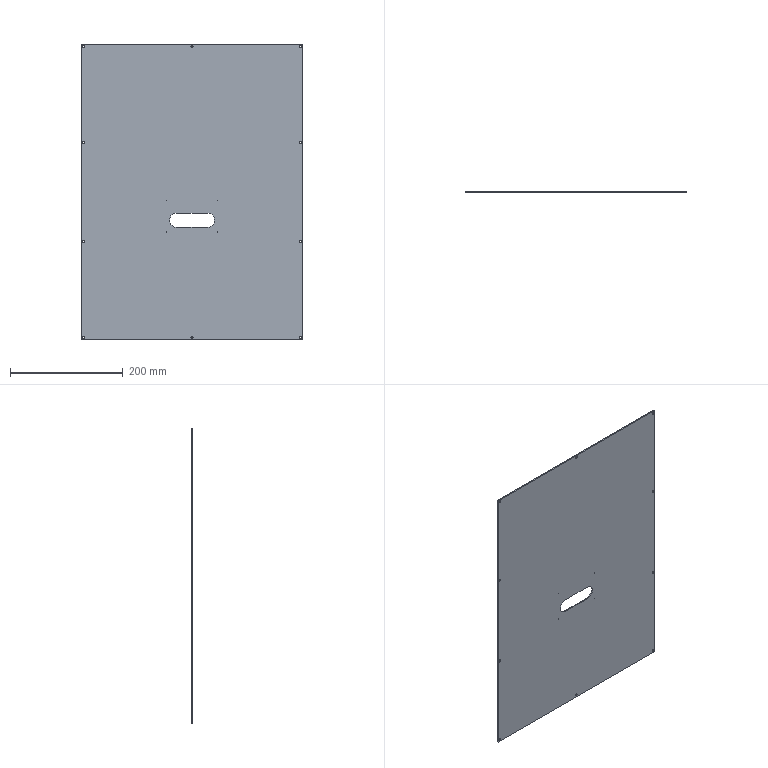Part | NX | features solid 2 | 1 solid | 39 faces | box 393 x 2 x 524 mm | volume 407875 mm3 | cylinder 31 | plane 8 | commonest cylinder face diameters 4 x20 1 x8 25 x3
STEP:
#1=CARTESIAN_POINT('',(-708.,-1585.,647.));
#2=VERTEX_POINT('',#1);
#3=CARTESIAN_POINT('',(-708.,-1587.,647.));
#4=VERTEX_POINT('',#3);
#5=CARTESIAN_POINT('',(-708.,-931.997,647.));
#6=DIRECTION('',(0.,-1.,0.));
#7=VECTOR('',#6,1000.);
#8=LINE('',#5,#7);
#9=EDGE_CURVE('',#2,#4,#8,.T.);
#10=ORIENTED_EDGE('',*,*,#9,.F.);
#11=CARTESIAN_POINT('',(-707.,-1585.,647.));
#12=VERTEX_POINT('',#11);
#13=CARTESIAN_POINT('',(-707.5,-1585.,647.));
#14=DIRECTION('',(0.,-1.,0.));
#15=DIRECTION('',(1.,0.,0.));
#16=AXIS2_PLACEMENT_3D('',#13,#14,#15);
#17=CIRCLE('',#16,0.5);
#18=EDGE_CURVE('',#12,#2,#17,.T.);
#19=ORIENTED_EDGE('',*,*,#18,.F.);
#20=CARTESIAN_POINT('',(-707.,-1587.,647.));
#21=VERTEX_POINT('',#20);
#22=CARTESIAN_POINT('',(-707.,-931.997,647.));
#23=DIRECTION('',(0.,-1.,0.));
#24=VECTOR('',#23,1000.);
#25=LINE('',#22,#24);
#26=EDGE_CURVE('',#21,#12,#25,.F.);
#27=ORIENTED_EDGE('',*,*,#26,.F.);
#28=CARTESIAN_POINT('',(-707.5,-1587.,647.));
#29=DIRECTION('',(0.,-1.,0.));
#30=DIRECTION('',(1.,0.,0.));
#31=AXIS2_PLACEMENT_3D('',#28,#29,#30);
#32=CIRCLE('',#31,0.5);
#33=EDGE_CURVE('',#21,#4,#32,.T.);
#34=ORIENTED_EDGE('',*,*,#33,.T.);
#35=EDGE_LOOP('',(#10,#19,#27,#34));
#36=FACE_BOUND('',#35,.T.);
#37=CARTESIAN_POINT('',(-707.5,-931.997,647.));
#38=DIRECTION('',(0.,-1.,0.));
#39=DIRECTION('',(1.,0.,0.));
#40=AXIS2_PLACEMENT_3D('',#37,#38,#39);
#41=CYLINDRICAL_SURFACE('',#40,0.5);
#42=ADVANCED_FACE('',(#36),#41,.F.);
#43=CARTESIAN_POINT('',(-618.,-1585.,647.));
#44=VERTEX_POINT('',#43);
#45=CARTESIAN_POINT('',(-618.,-1587.,647.));
#46=VERTEX_POINT('',#45);
#47=CARTESIAN_POINT('',(-618.,-931.997,647.));
#48=DIRECTION('',(0.,-1.,0.));
#49=VECTOR('',#48,1000.);
#50=LINE('',#47,#49);
#51=EDGE_CURVE('',#44,#46,#50,.T.);
#52=ORIENTED_EDGE('',*,*,#51,.F.);
#53=CARTESIAN_POINT('',(-617.,-1585.,647.));
#54=VERTEX_POINT('',#53);
#55=CARTESIAN_POINT('',(-617.5,-1585.,647.));
#56=DIRECTION('',(0.,-1.,0.));
#57=DIRECTION('',(1.,0.,0.));
#58=AXIS2_PLACEMENT_3D('',#55,#56,#57);
#59=CIRCLE('',#58,0.5);
#60=EDGE_CURVE('',#54,#44,#59,.T.);
#61=ORIENTED_EDGE('',*,*,#60,.F.);
#62=CARTESIAN_POINT('',(-617.,-1587.,647.));
#63=VERTEX_POINT('',#62);
#64=CARTESIAN_POINT('',(-617.,-931.997,647.));
#65=DIRECTION('',(0.,-1.,0.));
#66=VECTOR('',#65,1000.);
#67=LINE('',#64,#66);
#68=EDGE_CURVE('',#63,#54,#67,.F.);
#69=ORIENTED_EDGE('',*,*,#68,.F.);
#70=CARTESIAN_POINT('',(-617.5,-1587.,647.));
#71=DIRECTION('',(0.,-1.,0.));
#72=DIRECTION('',(1.,0.,0.));
#73=AXIS2_PLACEMENT_3D('',#70,#71,#72);
#74=CIRCLE('',#73,0.5);
#75=EDGE_CURVE('',#63,#46,#74,.T.);
#76=ORIENTED_EDGE('',*,*,#75,.T.);
#77=EDGE_LOOP('',(#52,#61,#69,#76));
#78=FACE_BOUND('',#77,.T.);
#79=CARTESIAN_POINT('',(-617.5,-931.997,647.));
#80=DIRECTION('',(0.,-1.,0.));
#81=DIRECTION('',(1.,0.,0.));
#82=AXIS2_PLACEMENT_3D('',#79,#80,#81);
#83=CYLINDRICAL_SURFACE('',#82,0.5);
#84=ADVANCED_FACE('',(#78),#83,.F.);
#85=CARTESIAN_POINT('',(-618.,-1587.,591.));
#86=VERTEX_POINT('',#85);
#87=CARTESIAN_POINT('',(-618.,-1585.,591.));
#88=VERTEX_POINT('',#87);
#89=CARTESIAN_POINT('',(-618.,-931.997,591.));
#90=DIRECTION('',(0.,-1.,0.));
#91=VECTOR('',#90,1000.);
#92=LINE('',#89,#91);
#93=EDGE_CURVE('',#86,#88,#92,.F.);
#94=ORIENTED_EDGE('',*,*,#93,.T.);
#95=CARTESIAN_POINT('',(-617.,-1585.,591.));
#96=VERTEX_POINT('',#95);
#97=CARTESIAN_POINT('',(-617.5,-1585.,591.));
#98=DIRECTION('',(0.,-1.,0.));
#99=DIRECTION('',(1.,0.,0.));
#100=AXIS2_PLACEMENT_3D('',#97,#98,#99);
#101=CIRCLE('',#100,0.5);
#102=EDGE_CURVE('',#96,#88,#101,.T.);
#103=ORIENTED_EDGE('',*,*,#102,.F.);
#104=CARTESIAN_POINT('',(-617.,-1587.,591.));
#105=VERTEX_POINT('',#104);
#106=CARTESIAN_POINT('',(-617.,-931.997,591.));
#107=DIRECTION('',(0.,-1.,0.));
#108=VECTOR('',#107,1000.);
#109=LINE('',#106,#108);
#110=EDGE_CURVE('',#96,#105,#109,.T.);
#111=ORIENTED_EDGE('',*,*,#110,.T.);
#112=CARTESIAN_POINT('',(-617.5,-1587.,591.));
#113=DIRECTION('',(0.,-1.,0.));
#114=DIRECTION('',(1.,0.,0.));
#115=AXIS2_PLACEMENT_3D('',#112,#113,#114);
#116=CIRCLE('',#115,0.5);
#117=EDGE_CURVE('',#105,#86,#116,.T.);
#118=ORIENTED_EDGE('',*,*,#117,.T.);
#119=EDGE_LOOP('',(#94,#103,#111,#118));
#120=FACE_BOUND('',#119,.T.);
#121=CARTESIAN_POINT('',(-617.5,-931.997,591.));
#122=DIRECTION('',(0.,-1.,0.));
#123=DIRECTION('',(1.,0.,0.));
#124=AXIS2_PLACEMENT_3D('',#121,#122,#123);
#125=CYLINDRICAL_SURFACE('',#124,0.5);
#126=ADVANCED_FACE('',(#120),#125,.F.);
#127=CARTESIAN_POINT('',(-708.,-1587.,591.));
#128=VERTEX_POINT('',#127);
#129=CARTESIAN_POINT('',(-708.,-1585.,591.));
#130=VERTEX_POINT('',#129);
#131=CARTESIAN_POINT('',(-708.,-931.997,591.));
#132=DIRECTION('',(0.,-1.,0.));
#133=VECTOR('',#132,1000.);
#134=LINE('',#131,#133);
#135=EDGE_CURVE('',#128,#130,#134,.F.);
#136=ORIENTED_EDGE('',*,*,#135,.T.);
#137=CARTESIAN_POINT('',(-707.,-1585.,591.));
#138=VERTEX_POINT('',#137);
#139=CARTESIAN_POINT('',(-707.5,-1585.,591.));
#140=DIRECTION('',(0.,-1.,0.));
#141=DIRECTION('',(1.,0.,0.));
#142=AXIS2_PLACEMENT_3D('',#139,#140,#141);
#143=CIRCLE('',#142,0.5);
#144=EDGE_CURVE('',#138,#130,#143,.T.);
#145=ORIENTED_EDGE('',*,*,#144,.F.);
#146=CARTESIAN_POINT('',(-707.,-1587.,591.));
#147=VERTEX_POINT('',#146);
#148=CARTESIAN_POINT('',(-707.,-931.997,591.));
#149=DIRECTION('',(0.,-1.,0.));
#150=VECTOR('',#149,1000.);
#151=LINE('',#148,#150);
#152=EDGE_CURVE('',#138,#147,#151,.T.);
#153=ORIENTED_EDGE('',*,*,#152,.T.);
#154=CARTESIAN_POINT('',(-707.5,-1587.,591.));
#155=DIRECTION('',(0.,-1.,0.));
#156=DIRECTION('',(1.,0.,0.));
#157=AXIS2_PLACEMENT_3D('',#154,#155,#156);
#158=CIRCLE('',#157,0.5);
#159=EDGE_CURVE('',#147,#128,#158,.T.);
#160=ORIENTED_EDGE('',*,*,#159,.T.);
#161=EDGE_LOOP('',(#136,#145,#153,#160));
#162=FACE_BOUND('',#161,.T.);
#163=CARTESIAN_POINT('',(-707.5,-931.997,591.));
#164=DIRECTION('',(0.,-1.,0.));
#165=DIRECTION('',(1.,0.,0.));
#166=AXIS2_PLACEMENT_3D('',#163,#164,#165);
#167=CYLINDRICAL_SURFACE('',#166,0.5);
#168=ADVANCED_FACE('',(#162),#167,.F.);
#169=CARTESIAN_POINT('',(-690.,-1587.,599.5));
#170=VERTEX_POINT('',#169);
#171=CARTESIAN_POINT('',(-635.,-1587.,599.5));
#172=VERTEX_POINT('',#171);
#173=CARTESIAN_POINT('',(-859.,-1587.,599.5));
#174=DIRECTION('',(1.,0.,0.));
#175=VECTOR('',#174,1000.);
#176=LINE('',#173,#175);
#177=EDGE_CURVE('',#170,#172,#176,.T.);
#178=ORIENTED_EDGE('',*,*,#177,.T.);
#179=CARTESIAN_POINT('',(-635.,-1585.,599.5));
#180=VERTEX_POINT('',#179);
#181=CARTESIAN_POINT('',(-635.,-2240.003,599.5));
#182=DIRECTION('',(0.,1.,0.));
#183=VECTOR('',#182,1000.);
#184=LINE('',#181,#183);
#185=EDGE_CURVE('',#172,#180,#184,.T.);
#186=ORIENTED_EDGE('',*,*,#185,.T.);
#187=CARTESIAN_POINT('',(-690.,-1585.,599.5));
#188=VERTEX_POINT('',#187);
#189=CARTESIAN_POINT('',(-635.,-1585.,599.5));
#190=DIRECTION('',(-1.,0.,0.));
#191=VECTOR('',#190,1000.);
#192=LINE('',#189,#191);
#193=EDGE_CURVE('',#180,#188,#192,.T.);
#194=ORIENTED_EDGE('',*,*,#193,.T.);
#195=CARTESIAN_POINT('',(-690.,-2240.003,599.5));
#196=DIRECTION('',(0.,1.,0.));
#197=VECTOR('',#196,1000.);
#198=LINE('',#195,#197);
#199=EDGE_CURVE('',#170,#188,#198,.T.);
#200=ORIENTED_EDGE('',*,*,#199,.F.);
#201=EDGE_LOOP('',(#178,#186,#194,#200));
#202=FACE_BOUND('',#201,.T.);
#203=CARTESIAN_POINT('',(-635.,-2240.003,599.5));
#204=DIRECTION('',(0.,0.,-1.));
#205=DIRECTION('',(0.,-1.,0.));
#206=AXIS2_PLACEMENT_3D('',#203,#204,#205);
#207=PLANE('',#206);
#208=ADVANCED_FACE('',(#202),#207,.F.);
#209=CARTESIAN_POINT('',(-635.,-1587.,624.5));
#210=VERTEX_POINT('',#209);
#211=CARTESIAN_POINT('',(-635.,-1587.,612.));
#212=DIRECTION('',(0.,-1.,0.));
#213=DIRECTION('',(1.,0.,0.));
#214=AXIS2_PLACEMENT_3D('',#211,#212,#213);
#215=CIRCLE('',#214,12.5);
#216=EDGE_CURVE('',#172,#210,#215,.T.);
#217=ORIENTED_EDGE('',*,*,#216,.T.);
#218=CARTESIAN_POINT('',(-635.,-1585.,624.5));
#219=VERTEX_POINT('',#218);
#220=CARTESIAN_POINT('',(-635.,-2240.003,624.5));
#221=DIRECTION('',(0.,1.,0.));
#222=VECTOR('',#221,1000.);
#223=LINE('',#220,#222);
#224=EDGE_CURVE('',#210,#219,#223,.T.);
#225=ORIENTED_EDGE('',*,*,#224,.T.);
#226=CARTESIAN_POINT('',(-635.,-1585.,612.));
#227=DIRECTION('',(0.,1.,0.));
#228=DIRECTION('',(-1.,0.,0.));
#229=AXIS2_PLACEMENT_3D('',#226,#227,#228);
#230=CIRCLE('',#229,12.5);
#231=EDGE_CURVE('',#219,#180,#230,.T.);
#232=ORIENTED_EDGE('',*,*,#231,.T.);
#233=ORIENTED_EDGE('',*,*,#185,.F.);
#234=EDGE_LOOP('',(#217,#225,#232,#233));
#235=FACE_BOUND('',#234,.T.);
#236=CARTESIAN_POINT('',(-635.,-2240.003,612.));
#237=DIRECTION('',(0.,1.,0.));
#238=DIRECTION('',(-1.,0.,0.));
#239=AXIS2_PLACEMENT_3D('',#236,#237,#238);
#240=CYLINDRICAL_SURFACE('',#239,12.5);
#241=ADVANCED_FACE('',(#235),#240,.F.);
#242=CARTESIAN_POINT('',(-690.,-1587.,624.5));
#243=VERTEX_POINT('',#242);
#244=CARTESIAN_POINT('',(-859.,-1587.,624.5));
#245=DIRECTION('',(-1.,0.,0.));
#246=VECTOR('',#245,1000.);
#247=LINE('',#244,#246);
#248=EDGE_CURVE('',#210,#243,#247,.T.);
#249=ORIENTED_EDGE('',*,*,#248,.T.);
#250=CARTESIAN_POINT('',(-690.,-1585.,624.5));
#251=VERTEX_POINT('',#250);
#252=CARTESIAN_POINT('',(-690.,-2240.003,624.5));
#253=DIRECTION('',(0.,1.,0.));
#254=VECTOR('',#253,1000.);
#255=LINE('',#252,#254);
#256=EDGE_CURVE('',#243,#251,#255,.T.);
#257=ORIENTED_EDGE('',*,*,#256,.T.);
#258=CARTESIAN_POINT('',(-635.,-1585.,624.5));
#259=DIRECTION('',(1.,0.,0.));
#260=VECTOR('',#259,1000.);
#261=LINE('',#258,#260);
#262=EDGE_CURVE('',#251,#219,#261,.T.);
#263=ORIENTED_EDGE('',*,*,#262,.T.);
#264=ORIENTED_EDGE('',*,*,#224,.F.);
#265=EDGE_LOOP('',(#249,#257,#263,#264));
#266=FACE_BOUND('',#265,.T.);
#267=CARTESIAN_POINT('',(-635.,-2240.003,624.5));
#268=DIRECTION('',(0.,0.,1.));
#269=DIRECTION('',(1.,0.,0.));
#270=AXIS2_PLACEMENT_3D('',#267,#268,#269);
#271=PLANE('',#270);
#272=ADVANCED_FACE('',(#266),#271,.F.);
#273=CARTESIAN_POINT('',(-702.5,-1587.,612.));
#274=VERTEX_POINT('',#273);
#275=CARTESIAN_POINT('',(-702.5,-1585.,612.));
#276=VERTEX_POINT('',#275);
#277=CARTESIAN_POINT('',(-702.5,-2240.003,612.));
#278=DIRECTION('',(0.,1.,0.));
#279=VECTOR('',#278,1000.);
#280=LINE('',#277,#279);
#281=EDGE_CURVE('',#274,#276,#280,.T.);
#282=ORIENTED_EDGE('',*,*,#281,.F.);
#283=CARTESIAN_POINT('',(-690.,-1587.,612.));
#284=DIRECTION('',(0.,-1.,0.));
#285=DIRECTION('',(1.,0.,0.));
#286=AXIS2_PLACEMENT_3D('',#283,#284,#285);
#287=CIRCLE('',#286,12.5);
#288=EDGE_CURVE('',#274,#170,#287,.T.);
#289=ORIENTED_EDGE('',*,*,#288,.T.);
#290=ORIENTED_EDGE('',*,*,#199,.T.);
#291=CARTESIAN_POINT('',(-690.,-1585.,612.));
#292=DIRECTION('',(0.,1.,0.));
#293=DIRECTION('',(1.,0.,0.));
#294=AXIS2_PLACEMENT_3D('',#291,#292,#293);
#295=CIRCLE('',#294,12.5);
#296=EDGE_CURVE('',#188,#276,#295,.T.);
#297=ORIENTED_EDGE('',*,*,#296,.T.);
#298=EDGE_LOOP('',(#282,#289,#290,#297));
#299=FACE_BOUND('',#298,.T.);
#300=CARTESIAN_POINT('',(-690.,-2240.003,612.));
#301=DIRECTION('',(0.,1.,0.));
#302=DIRECTION('',(-1.,0.,0.));
#303=AXIS2_PLACEMENT_3D('',#300,#301,#302);
#304=CYLINDRICAL_SURFACE('',#303,12.5);
#305=ADVANCED_FACE('',(#299),#304,.F.);
#306=CARTESIAN_POINT('',(-472.,-1585.,574.));
#307=VERTEX_POINT('',#306);
#308=CARTESIAN_POINT('',(-472.,-1587.,574.));
#309=VERTEX_POINT('',#308);
#310=CARTESIAN_POINT('',(-472.,-931.997,574.));
#311=DIRECTION('',(0.,-1.,0.));
#312=VECTOR('',#311,1000.);
#313=LINE('',#310,#312);
#314=EDGE_CURVE('',#307,#309,#313,.T.);
#315=ORIENTED_EDGE('',*,*,#314,.F.);
#316=CARTESIAN_POINT('',(-468.,-1585.,574.));
#317=VERTEX_POINT('',#316);
#318=CARTESIAN_POINT('',(-470.,-1585.,574.));
#319=DIRECTION('',(0.,-1.,0.));
#320=DIRECTION('',(1.,0.,0.));
#321=AXIS2_PLACEMENT_3D('',#318,#319,#320);
#322=CIRCLE('',#321,2.);
#323=EDGE_CURVE('',#317,#307,#322,.T.);
#324=ORIENTED_EDGE('',*,*,#323,.F.);
#325=CARTESIAN_POINT('',(-468.,-1587.,574.));
#326=VERTEX_POINT('',#325);
#327=CARTESIAN_POINT('',(-468.,-931.997,574.));
#328=DIRECTION('',(0.,-1.,0.));
#329=VECTOR('',#328,1000.);
#330=LINE('',#327,#329);
#331=EDGE_CURVE('',#326,#317,#330,.F.);
#332=ORIENTED_EDGE('',*,*,#331,.F.);
#333=CARTESIAN_POINT('',(-470.,-1587.,574.));
#334=DIRECTION('',(0.,-1.,0.));
#335=DIRECTION('',(1.,0.,0.));
#336=AXIS2_PLACEMENT_3D('',#333,#334,#335);
#337=CIRCLE('',#336,2.);
#338=EDGE_CURVE('',#326,#309,#337,.T.);
#339=ORIENTED_EDGE('',*,*,#338,.T.);
#340=EDGE_LOOP('',(#315,#324,#332,#339));
#341=FACE_BOUND('',#340,.T.);
#342=CARTESIAN_POINT('',(-470.,-931.997,574.));
#343=DIRECTION('',(0.,-1.,0.));
#344=DIRECTION('',(1.,0.,0.));
#345=AXIS2_PLACEMENT_3D('',#342,#343,#344);
#346=CYLINDRICAL_SURFACE('',#345,2.);
#347=ADVANCED_FACE('',(#341),#346,.F.);
#348=CARTESIAN_POINT('',(-857.,-1587.,574.));
#349=VERTEX_POINT('',#348);
#350=CARTESIAN_POINT('',(-857.,-1585.,574.));
#351=VERTEX_POINT('',#350);
#352=CARTESIAN_POINT('',(-857.,-931.997,574.));
#353=DIRECTION('',(0.,-1.,0.));
#354=VECTOR('',#353,1000.);
#355=LINE('',#352,#354);
#356=EDGE_CURVE('',#349,#351,#355,.F.);
#357=ORIENTED_EDGE('',*,*,#356,.T.);
#358=CARTESIAN_POINT('',(-853.,-1585.,574.));
#359=VERTEX_POINT('',#358);
#360=CARTESIAN_POINT('',(-855.,-1585.,574.));
#361=DIRECTION('',(0.,-1.,0.));
#362=DIRECTION('',(1.,0.,0.));
#363=AXIS2_PLACEMENT_3D('',#360,#361,#362);
#364=CIRCLE('',#363,2.);
#365=EDGE_CURVE('',#359,#351,#364,.T.);
#366=ORIENTED_EDGE('',*,*,#365,.F.);
#367=CARTESIAN_POINT('',(-853.,-1587.,574.));
#368=VERTEX_POINT('',#367);
#369=CARTESIAN_POINT('',(-853.,-931.997,574.));
#370=DIRECTION('',(0.,-1.,0.));
#371=VECTOR('',#370,1000.);
#372=LINE('',#369,#371);
#373=EDGE_CURVE('',#359,#368,#372,.T.);
#374=ORIENTED_EDGE('',*,*,#373,.T.);
#375=CARTESIAN_POINT('',(-855.,-1587.,574.));
#376=DIRECTION('',(0.,-1.,0.));
#377=DIRECTION('',(1.,0.,0.));
#378=AXIS2_PLACEMENT_3D('',#375,#376,#377);
#379=CIRCLE('',#378,2.);
#380=EDGE_CURVE('',#368,#349,#379,.T.);
#381=ORIENTED_EDGE('',*,*,#380,.T.);
#382=EDGE_LOOP('',(#357,#366,#374,#381));
#383=FACE_BOUND('',#382,.T.);
#384=CARTESIAN_POINT('',(-855.,-931.997,574.));
#385=DIRECTION('',(0.,-1.,0.));
#386=DIRECTION('',(1.,0.,0.));
#387=AXIS2_PLACEMENT_3D('',#384,#385,#386);
#388=CYLINDRICAL_SURFACE('',#387,2.);
#389=ADVANCED_FACE('',(#383),#388,.F.);
#390=CARTESIAN_POINT('',(-857.,-1587.,920.));
#391=VERTEX_POINT('',#390);
#392=CARTESIAN_POINT('',(-857.,-1585.,920.));
#393=VERTEX_POINT('',#392);
#394=CARTESIAN_POINT('',(-857.,-931.997,920.));
#395=DIRECTION('',(0.,-1.,0.));
#396=VECTOR('',#395,1000.);
#397=LINE('',#394,#396);
#398=EDGE_CURVE('',#391,#393,#397,.F.);
#399=ORIENTED_EDGE('',*,*,#398,.T.);
#400=CARTESIAN_POINT('',(-853.,-1585.,920.));
#401=VERTEX_POINT('',#400);
#402=CARTESIAN_POINT('',(-855.,-1585.,920.));
#403=DIRECTION('',(0.,-1.,0.));
#404=DIRECTION('',(1.,0.,0.));
#405=AXIS2_PLACEMENT_3D('',#402,#403,#404);
#406=CIRCLE('',#405,2.);
#407=EDGE_CURVE('',#401,#393,#406,.T.);
#408=ORIENTED_EDGE('',*,*,#407,.F.);
#409=CARTESIAN_POINT('',(-853.,-1587.,920.));
#410=VERTEX_POINT('',#409);
#411=CARTESIAN_POINT('',(-853.,-931.997,920.));
#412=DIRECTION('',(0.,-1.,0.));
#413=VECTOR('',#412,1000.);
#414=LINE('',#411,#413);
#415=EDGE_CURVE('',#401,#410,#414,.T.);
#416=ORIENTED_EDGE('',*,*,#415,.T.);
#417=CARTESIAN_POINT('',(-855.,-1587.,920.));
#418=DIRECTION('',(0.,-1.,0.));
#419=DIRECTION('',(1.,0.,0.));
#420=AXIS2_PLACEMENT_3D('',#417,#418,#419);
#421=CIRCLE('',#420,2.);
#422=EDGE_CURVE('',#410,#391,#421,.T.);
#423=ORIENTED_EDGE('',*,*,#422,.T.);
#424=EDGE_LOOP('',(#399,#408,#416,#423));
#425=FACE_BOUND('',#424,.T.);
#426=CARTESIAN_POINT('',(-855.,-931.997,920.));
#427=DIRECTION('',(0.,-1.,0.));
#428=DIRECTION('',(1.,0.,0.));
#429=AXIS2_PLACEMENT_3D('',#426,#427,#428);
#430=CYLINDRICAL_SURFACE('',#429,2.);
#431=ADVANCED_FACE('',(#425),#430,.F.);
#432=CARTESIAN_POINT('',(-857.,-1585.,750.));
#433=VERTEX_POINT('',#432);
#434=CARTESIAN_POINT('',(-857.,-1587.,750.));
#435=VERTEX_POINT('',#434);
#436=CARTESIAN_POINT('',(-857.,-931.997,750.));
#437=DIRECTION('',(0.,-1.,0.));
#438=VECTOR('',#437,1000.);
#439=LINE('',#436,#438);
#440=EDGE_CURVE('',#433,#435,#439,.T.);
#441=ORIENTED_EDGE('',*,*,#440,.F.);
#442=CARTESIAN_POINT('',(-853.,-1585.,750.));
#443=VERTEX_POINT('',#442);
#444=CARTESIAN_POINT('',(-855.,-1585.,750.));
#445=DIRECTION('',(0.,-1.,0.));
#446=DIRECTION('',(1.,0.,0.));
#447=AXIS2_PLACEMENT_3D('',#444,#445,#446);
#448=CIRCLE('',#447,2.);
#449=EDGE_CURVE('',#443,#433,#448,.T.);
#450=ORIENTED_EDGE('',*,*,#449,.F.);
#451=CARTESIAN_POINT('',(-853.,-1587.,750.));
#452=VERTEX_POINT('',#451);
#453=CARTESIAN_POINT('',(-853.,-931.997,750.));
#454=DIRECTION('',(0.,-1.,0.));
#455=VECTOR('',#454,1000.);
#456=LINE('',#453,#455);
#457=EDGE_CURVE('',#452,#443,#456,.F.);
#458=ORIENTED_EDGE('',*,*,#457,.F.);
#459=CARTESIAN_POINT('',(-855.,-1587.,750.));
#460=DIRECTION('',(0.,-1.,0.));
#461=DIRECTION('',(1.,0.,0.));
#462=AXIS2_PLACEMENT_3D('',#459,#460,#461);
#463=CIRCLE('',#462,2.);
#464=EDGE_CURVE('',#452,#435,#463,.T.);
#465=ORIENTED_EDGE('',*,*,#464,.T.);
#466=EDGE_LOOP('',(#441,#450,#458,#465));
#467=FACE_BOUND('',#466,.T.);
#468=CARTESIAN_POINT('',(-855.,-931.997,750.));
#469=DIRECTION('',(0.,-1.,0.));
#470=DIRECTION('',(1.,0.,0.));
#471=AXIS2_PLACEMENT_3D('',#468,#469,#470);
#472=CYLINDRICAL_SURFACE('',#471,2.);
#473=ADVANCED_FACE('',(#467),#472,.F.);
#474=CARTESIAN_POINT('',(-857.,-1587.,404.));
#475=VERTEX_POINT('',#474);
#476=CARTESIAN_POINT('',(-857.,-1585.,404.));
#477=VERTEX_POINT('',#476);
#478=CARTESIAN_POINT('',(-857.,-931.997,404.));
#479=DIRECTION('',(0.,-1.,0.));
#480=VECTOR('',#479,1000.);
#481=LINE('',#478,#480);
#482=EDGE_CURVE('',#475,#477,#481,.F.);
#483=ORIENTED_EDGE('',*,*,#482,.T.);
#484=CARTESIAN_POINT('',(-853.,-1585.,404.));
#485=VERTEX_POINT('',#484);
#486=CARTESIAN_POINT('',(-855.,-1585.,404.));
#487=DIRECTION('',(0.,-1.,0.));
#488=DIRECTION('',(1.,0.,0.));
#489=AXIS2_PLACEMENT_3D('',#486,#487,#488);
#490=CIRCLE('',#489,2.);
#491=EDGE_CURVE('',#485,#477,#490,.T.);
#492=ORIENTED_EDGE('',*,*,#491,.F.);
#493=CARTESIAN_POINT('',(-853.,-1587.,404.));
#494=VERTEX_POINT('',#493);
#495=CARTESIAN_POINT('',(-853.,-931.997,404.));
#496=DIRECTION('',(0.,-1.,0.));
#497=VECTOR('',#496,1000.);
#498=LINE('',#495,#497);
#499=EDGE_CURVE('',#485,#494,#498,.T.);
#500=ORIENTED_EDGE('',*,*,#499,.T.);
#501=CARTESIAN_POINT('',(-855.,-1587.,404.));
#502=DIRECTION('',(0.,-1.,0.));
#503=DIRECTION('',(1.,0.,0.));
#504=AXIS2_PLACEMENT_3D('',#501,#502,#503);
#505=CIRCLE('',#504,2.);
#506=EDGE_CURVE('',#494,#475,#505,.T.);
#507=ORIENTED_EDGE('',*,*,#506,.T.);
#508=EDGE_LOOP('',(#483,#492,#500,#507));
#509=FACE_BOUND('',#508,.T.);
#510=CARTESIAN_POINT('',(-855.,-931.997,404.));
#511=DIRECTION('',(0.,-1.,0.));
#512=DIRECTION('',(1.,0.,0.));
#513=AXIS2_PLACEMENT_3D('',#510,#511,#512);
#514=CYLINDRICAL_SURFACE('',#513,2.);
#515=ADVANCED_FACE('',(#509),#514,.F.);
#516=CARTESIAN_POINT('',(-664.5,-1587.,404.));
#517=VERTEX_POINT('',#516);
#518=CARTESIAN_POINT('',(-664.5,-1585.,404.));
#519=VERTEX_POINT('',#518);
#520=CARTESIAN_POINT('',(-664.5,-931.997,404.));
#521=DIRECTION('',(0.,-1.,0.));
#522=VECTOR('',#521,1000.);
#523=LINE('',#520,#522);
#524=EDGE_CURVE('',#517,#519,#523,.F.);
#525=ORIENTED_EDGE('',*,*,#524,.T.);
#526=CARTESIAN_POINT('',(-660.5,-1585.,404.));
#527=VERTEX_POINT('',#526);
#528=CARTESIAN_POINT('',(-662.5,-1585.,404.));
#529=DIRECTION('',(0.,-1.,0.));
#530=DIRECTION('',(1.,0.,0.));
#531=AXIS2_PLACEMENT_3D('',#528,#529,#530);
#532=CIRCLE('',#531,2.);
#533=EDGE_CURVE('',#527,#519,#532,.T.);
#534=ORIENTED_EDGE('',*,*,#533,.F.);
#535=CARTESIAN_POINT('',(-660.5,-1587.,404.));
#536=VERTEX_POINT('',#535);
#537=CARTESIAN_POINT('',(-660.5,-931.997,404.));
#538=DIRECTION('',(0.,-1.,0.));
#539=VECTOR('',#538,1000.);
#540=LINE('',#537,#539);
#541=EDGE_CURVE('',#527,#536,#540,.T.);
#542=ORIENTED_EDGE('',*,*,#541,.T.);
#543=CARTESIAN_POINT('',(-662.5,-1587.,404.));
#544=DIRECTION('',(0.,-1.,0.));
#545=DIRECTION('',(1.,0.,0.));
#546=AXIS2_PLACEMENT_3D('',#543,#544,#545);
#547=CIRCLE('',#546,2.);
#548=EDGE_CURVE('',#536,#517,#547,.T.);
#549=ORIENTED_EDGE('',*,*,#548,.T.);
#550=EDGE_LOOP('',(#525,#534,#542,#549));
#551=FACE_BOUND('',#550,.T.);
#552=CARTESIAN_POINT('',(-662.5,-931.997,404.));
#553=DIRECTION('',(0.,-1.,0.));
#554=DIRECTION('',(1.,0.,0.));
#555=AXIS2_PLACEMENT_3D('',#552,#553,#554);
#556=CYLINDRICAL_SURFACE('',#555,2.);
#557=ADVANCED_FACE('',(#551),#556,.F.);
#558=CARTESIAN_POINT('',(-472.,-1585.,404.));
#559=VERTEX_POINT('',#558);
#560=CARTESIAN_POINT('',(-472.,-1587.,404.));
#561=VERTEX_POINT('',#560);
#562=CARTESIAN_POINT('',(-472.,-931.997,404.));
#563=DIRECTION('',(0.,-1.,0.));
#564=VECTOR('',#563,1000.);
#565=LINE('',#562,#564);
#566=EDGE_CURVE('',#559,#561,#565,.T.);
#567=ORIENTED_EDGE('',*,*,#566,.F.);
#568=CARTESIAN_POINT('',(-468.,-1585.,404.));
#569=VERTEX_POINT('',#568);
#570=CARTESIAN_POINT('',(-470.,-1585.,404.));
#571=DIRECTION('',(0.,-1.,0.));
#572=DIRECTION('',(1.,0.,0.));
#573=AXIS2_PLACEMENT_3D('',#570,#571,#572);
#574=CIRCLE('',#573,2.);
#575=EDGE_CURVE('',#569,#559,#574,.T.);
#576=ORIENTED_EDGE('',*,*,#575,.F.);
#577=CARTESIAN_POINT('',(-468.,-1587.,404.));
#578=VERTEX_POINT('',#577);
#579=CARTESIAN_POINT('',(-468.,-931.997,404.));
#580=DIRECTION('',(0.,-1.,0.));
#581=VECTOR('',#580,1000.);
#582=LINE('',#579,#581);
#583=EDGE_CURVE('',#578,#569,#582,.F.);
#584=ORIENTED_EDGE('',*,*,#583,.F.);
#585=CARTESIAN_POINT('',(-470.,-1587.,404.));
#586=DIRECTION('',(0.,-1.,0.));
#587=DIRECTION('',(1.,0.,0.));
#588=AXIS2_PLACEMENT_3D('',#585,#586,#587);
#589=CIRCLE('',#588,2.);
#590=EDGE_CURVE('',#578,#561,#589,.T.);
#591=ORIENTED_EDGE('',*,*,#590,.T.);
#592=EDGE_LOOP('',(#567,#576,#584,#591));
#593=FACE_BOUND('',#592,.T.);
#594=CARTESIAN_POINT('',(-470.,-931.997,404.));
#595=DIRECTION('',(0.,-1.,0.));
#596=DIRECTION('',(1.,0.,0.));
#597=AXIS2_PLACEMENT_3D('',#594,#595,#596);
#598=CYLINDRICAL_SURFACE('',#597,2.);
#599=ADVANCED_FACE('',(#593),#598,.F.);
#600=CARTESIAN_POINT('',(-472.,-1585.,750.));
#601=VERTEX_POINT('',#600);
#602=CARTESIAN_POINT('',(-472.,-1587.,750.));
#603=VERTEX_POINT('',#602);
#604=CARTESIAN_POINT('',(-472.,-931.997,750.));
#605=DIRECTION('',(0.,-1.,0.));
#606=VECTOR('',#605,1000.);
#607=LINE('',#604,#606);
#608=EDGE_CURVE('',#601,#603,#607,.T.);
#609=ORIENTED_EDGE('',*,*,#608,.F.);
#610=CARTESIAN_POINT('',(-468.,-1585.,750.));
#611=VERTEX_POINT('',#610);
#612=CARTESIAN_POINT('',(-470.,-1585.,750.));
#613=DIRECTION('',(0.,-1.,0.));
#614=DIRECTION('',(1.,0.,0.));
#615=AXIS2_PLACEMENT_3D('',#612,#613,#614);
#616=CIRCLE('',#615,2.);
#617=EDGE_CURVE('',#611,#601,#616,.T.);
#618=ORIENTED_EDGE('',*,*,#617,.F.);
#619=CARTESIAN_POINT('',(-468.,-1587.,750.));
#620=VERTEX_POINT('',#619);
#621=CARTESIAN_POINT('',(-468.,-931.997,750.));
#622=DIRECTION('',(0.,-1.,0.));
#623=VECTOR('',#622,1000.);
#624=LINE('',#621,#623);
#625=EDGE_CURVE('',#620,#611,#624,.F.);
#626=ORIENTED_EDGE('',*,*,#625,.F.);
#627=CARTESIAN_POINT('',(-470.,-1587.,750.));
#628=DIRECTION('',(0.,-1.,0.));
#629=DIRECTION('',(1.,0.,0.));
#630=AXIS2_PLACEMENT_3D('',#627,#628,#629);
#631=CIRCLE('',#630,2.);
#632=EDGE_CURVE('',#620,#603,#631,.T.);
#633=ORIENTED_EDGE('',*,*,#632,.T.);
#634=EDGE_LOOP('',(#609,#618,#626,#633));
#635=FACE_BOUND('',#634,.T.);
#636=CARTESIAN_POINT('',(-470.,-931.997,750.));
#637=DIRECTION('',(0.,-1.,0.));
#638=DIRECTION('',(1.,0.,0.));
#639=AXIS2_PLACEMENT_3D('',#636,#637,#638);
#640=CYLINDRICAL_SURFACE('',#639,2.);
#641=ADVANCED_FACE('',(#635),#640,.F.);
#642=CARTESIAN_POINT('',(-472.,-1585.,920.));
#643=VERTEX_POINT('',#642);
#644=CARTESIAN_POINT('',(-472.,-1587.,920.));
#645=VERTEX_POINT('',#644);
#646=CARTESIAN_POINT('',(-472.,-931.997,920.));
#647=DIRECTION('',(0.,-1.,0.));
#648=VECTOR('',#647,1000.);
#649=LINE('',#646,#648);
#650=EDGE_CURVE('',#643,#645,#649,.T.);
#651=ORIENTED_EDGE('',*,*,#650,.F.);
#652=CARTESIAN_POINT('',(-468.,-1585.,920.));
#653=VERTEX_POINT('',#652);
#654=CARTESIAN_POINT('',(-470.,-1585.,920.));
#655=DIRECTION('',(0.,-1.,0.));
#656=DIRECTION('',(1.,0.,0.));
#657=AXIS2_PLACEMENT_3D('',#654,#655,#656);
#658=CIRCLE('',#657,2.);
#659=EDGE_CURVE('',#653,#643,#658,.T.);
#660=ORIENTED_EDGE('',*,*,#659,.F.);
#661=CARTESIAN_POINT('',(-468.,-1587.,920.));
#662=VERTEX_POINT('',#661);
#663=CARTESIAN_POINT('',(-468.,-931.997,920.));
#664=DIRECTION('',(0.,-1.,0.));
#665=VECTOR('',#664,1000.);
#666=LINE('',#663,#665);
#667=EDGE_CURVE('',#662,#653,#666,.F.);
#668=ORIENTED_EDGE('',*,*,#667,.F.);
#669=CARTESIAN_POINT('',(-470.,-1587.,920.));
#670=DIRECTION('',(0.,-1.,0.));
#671=DIRECTION('',(1.,0.,0.));
#672=AXIS2_PLACEMENT_3D('',#669,#670,#671);
#673=CIRCLE('',#672,2.);
#674=EDGE_CURVE('',#662,#645,#673,.T.);
#675=ORIENTED_EDGE('',*,*,#674,.T.);
#676=EDGE_LOOP('',(#651,#660,#668,#675));
#677=FACE_BOUND('',#676,.T.);
#678=CARTESIAN_POINT('',(-470.,-931.997,920.));
#679=DIRECTION('',(0.,-1.,0.));
#680=DIRECTION('',(1.,0.,0.));
#681=AXIS2_PLACEMENT_3D('',#678,#679,#680);
#682=CYLINDRICAL_SURFACE('',#681,2.);
#683=ADVANCED_FACE('',(#677),#682,.F.);
#684=CARTESIAN_POINT('',(-664.5,-1585.,920.));
#685=VERTEX_POINT('',#684);
#686=CARTESIAN_POINT('',(-664.5,-1587.,920.));
#687=VERTEX_POINT('',#686);
#688=CARTESIAN_POINT('',(-664.5,-931.997,920.));
#689=DIRECTION('',(0.,-1.,0.));
#690=VECTOR('',#689,1000.);
#691=LINE('',#688,#690);
#692=EDGE_CURVE('',#685,#687,#691,.T.);
#693=ORIENTED_EDGE('',*,*,#692,.F.);
#694=CARTESIAN_POINT('',(-660.5,-1585.,920.));
#695=VERTEX_POINT('',#694);
#696=CARTESIAN_POINT('',(-662.5,-1585.,920.));
#697=DIRECTION('',(0.,-1.,0.));
#698=DIRECTION('',(1.,0.,0.));
#699=AXIS2_PLACEMENT_3D('',#696,#697,#698);
#700=CIRCLE('',#699,2.);
#701=EDGE_CURVE('',#695,#685,#700,.T.);
#702=ORIENTED_EDGE('',*,*,#701,.F.);
#703=CARTESIAN_POINT('',(-660.5,-1587.,920.));
#704=VERTEX_POINT('',#703);
#705=CARTESIAN_POINT('',(-660.5,-931.997,920.));
#706=DIRECTION('',(0.,-1.,0.));
#707=VECTOR('',#706,1000.);
#708=LINE('',#705,#707);
#709=EDGE_CURVE('',#704,#695,#708,.F.);
#710=ORIENTED_EDGE('',*,*,#709,.F.);
#711=CARTESIAN_POINT('',(-662.5,-1587.,920.));
#712=DIRECTION('',(0.,-1.,0.));
#713=DIRECTION('',(1.,0.,0.));
#714=AXIS2_PLACEMENT_3D('',#711,#712,#713);
#715=CIRCLE('',#714,2.);
#716=EDGE_CURVE('',#704,#687,#715,.T.);
#717=ORIENTED_EDGE('',*,*,#716,.T.);
#718=EDGE_LOOP('',(#693,#702,#710,#717));
#719=FACE_BOUND('',#718,.T.);
#720=CARTESIAN_POINT('',(-662.5,-931.997,920.));
#721=DIRECTION('',(0.,-1.,0.));
#722=DIRECTION('',(1.,0.,0.));
#723=AXIS2_PLACEMENT_3D('',#720,#721,#722);
#724=CYLINDRICAL_SURFACE('',#723,2.);
#725=ADVANCED_FACE('',(#719),#724,.F.);
#726=ORIENTED_EDGE('',*,*,#701,.T.);
#727=CARTESIAN_POINT('',(-662.5,-1585.,920.));
#728=DIRECTION('',(0.,-1.,0.));
#729=DIRECTION('',(1.,0.,0.));
#730=AXIS2_PLACEMENT_3D('',#727,#728,#729);
#731=CIRCLE('',#730,2.);
#732=EDGE_CURVE('',#685,#695,#731,.T.);
#733=ORIENTED_EDGE('',*,*,#732,.T.);
#734=EDGE_LOOP('',(#726,#733));
#735=FACE_BOUND('',#734,.T.);
#736=ORIENTED_EDGE('',*,*,#659,.T.);
#737=CARTESIAN_POINT('',(-470.,-1585.,920.));
#738=DIRECTION('',(0.,-1.,0.));
#739=DIRECTION('',(1.,0.,0.));
#740=AXIS2_PLACEMENT_3D('',#737,#738,#739);
#741=CIRCLE('',#740,2.);
#742=EDGE_CURVE('',#643,#653,#741,.T.);
#743=ORIENTED_EDGE('',*,*,#742,.T.);
#744=EDGE_LOOP('',(#736,#743));
#745=FACE_BOUND('',#744,.T.);
#746=ORIENTED_EDGE('',*,*,#617,.T.);
#747=CARTESIAN_POINT('',(-470.,-1585.,750.));
#748=DIRECTION('',(0.,-1.,0.));
#749=DIRECTION('',(1.,0.,0.));
#750=AXIS2_PLACEMENT_3D('',#747,#748,#749);
#751=CIRCLE('',#750,2.);
#752=EDGE_CURVE('',#601,#611,#751,.T.);
#753=ORIENTED_EDGE('',*,*,#752,.T.);
#754=EDGE_LOOP('',(#746,#753));
#755=FACE_BOUND('',#754,.T.);
#756=ORIENTED_EDGE('',*,*,#575,.T.);
#757=CARTESIAN_POINT('',(-470.,-1585.,404.));
#758=DIRECTION('',(0.,-1.,0.));
#759=DIRECTION('',(1.,0.,0.));
#760=AXIS2_PLACEMENT_3D('',#757,#758,#759);
#761=CIRCLE('',#760,2.);
#762=EDGE_CURVE('',#559,#569,#761,.T.);
#763=ORIENTED_EDGE('',*,*,#762,.T.);
#764=EDGE_LOOP('',(#756,#763));
#765=FACE_BOUND('',#764,.T.);
#766=ORIENTED_EDGE('',*,*,#533,.T.);
#767=CARTESIAN_POINT('',(-662.5,-1585.,404.));
#768=DIRECTION('',(0.,-1.,0.));
#769=DIRECTION('',(1.,0.,0.));
#770=AXIS2_PLACEMENT_3D('',#767,#768,#769);
#771=CIRCLE('',#770,2.);
#772=EDGE_CURVE('',#519,#527,#771,.T.);
#773=ORIENTED_EDGE('',*,*,#772,.T.);
#774=EDGE_LOOP('',(#766,#773));
#775=FACE_BOUND('',#774,.T.);
#776=ORIENTED_EDGE('',*,*,#491,.T.);
#777=CARTESIAN_POINT('',(-855.,-1585.,404.));
#778=DIRECTION('',(0.,-1.,0.));
#779=DIRECTION('',(1.,0.,0.));
#780=AXIS2_PLACEMENT_3D('',#777,#778,#779);
#781=CIRCLE('',#780,2.);
#782=EDGE_CURVE('',#477,#485,#781,.T.);
#783=ORIENTED_EDGE('',*,*,#782,.T.);
#784=EDGE_LOOP('',(#776,#783));
#785=FACE_BOUND('',#784,.T.);
#786=ORIENTED_EDGE('',*,*,#449,.T.);
#787=CARTESIAN_POINT('',(-855.,-1585.,750.));
#788=DIRECTION('',(0.,-1.,0.));
#789=DIRECTION('',(1.,0.,0.));
#790=AXIS2_PLACEMENT_3D('',#787,#788,#789);
#791=CIRCLE('',#790,2.);
#792=EDGE_CURVE('',#433,#443,#791,.T.);
#793=ORIENTED_EDGE('',*,*,#792,.T.);
#794=EDGE_LOOP('',(#786,#793));
#795=FACE_BOUND('',#794,.T.);
#796=ORIENTED_EDGE('',*,*,#407,.T.);
#797=CARTESIAN_POINT('',(-855.,-1585.,920.));
#798=DIRECTION('',(0.,-1.,0.));
#799=DIRECTION('',(1.,0.,0.));
#800=AXIS2_PLACEMENT_3D('',#797,#798,#799);
#801=CIRCLE('',#800,2.);
#802=EDGE_CURVE('',#393,#401,#801,.T.);
#803=ORIENTED_EDGE('',*,*,#802,.T.);
#804=EDGE_LOOP('',(#796,#803));
#805=FACE_BOUND('',#804,.T.);
#806=ORIENTED_EDGE('',*,*,#365,.T.);
#807=CARTESIAN_POINT('',(-855.,-1585.,574.));
#808=DIRECTION('',(0.,-1.,0.));
#809=DIRECTION('',(1.,0.,0.));
#810=AXIS2_PLACEMENT_3D('',#807,#808,#809);
#811=CIRCLE('',#810,2.);
#812=EDGE_CURVE('',#351,#359,#811,.T.);
#813=ORIENTED_EDGE('',*,*,#812,.T.);
#814=EDGE_LOOP('',(#806,#813));
#815=FACE_BOUND('',#814,.T.);
#816=ORIENTED_EDGE('',*,*,#323,.T.);
#817=CARTESIAN_POINT('',(-470.,-1585.,574.));
#818=DIRECTION('',(0.,-1.,0.));
#819=DIRECTION('',(1.,0.,0.));
#820=AXIS2_PLACEMENT_3D('',#817,#818,#819);
#821=CIRCLE('',#820,2.);
#822=EDGE_CURVE('',#307,#317,#821,.T.);
#823=ORIENTED_EDGE('',*,*,#822,.T.);
#824=EDGE_LOOP('',(#816,#823));
#825=FACE_BOUND('',#824,.T.);
#826=ORIENTED_EDGE('',*,*,#262,.F.);
#827=CARTESIAN_POINT('',(-690.,-1585.,612.));
#828=DIRECTION('',(0.,1.,0.));
#829=DIRECTION('',(1.,0.,0.));
#830=AXIS2_PLACEMENT_3D('',#827,#828,#829);
#831=CIRCLE('',#830,12.5);
#832=EDGE_CURVE('',#276,#251,#831,.T.);
#833=ORIENTED_EDGE('',*,*,#832,.F.);
#834=ORIENTED_EDGE('',*,*,#296,.F.);
#835=ORIENTED_EDGE('',*,*,#193,.F.);
#836=ORIENTED_EDGE('',*,*,#231,.F.);
#837=EDGE_LOOP('',(#826,#833,#834,#835,#836));
#838=FACE_BOUND('',#837,.T.);
#839=ORIENTED_EDGE('',*,*,#144,.T.);
#840=CARTESIAN_POINT('',(-707.5,-1585.,591.));
#841=DIRECTION('',(0.,-1.,0.));
#842=DIRECTION('',(1.,0.,0.));
#843=AXIS2_PLACEMENT_3D('',#840,#841,#842);
#844=CIRCLE('',#843,0.5);
#845=EDGE_CURVE('',#130,#138,#844,.T.);
#846=ORIENTED_EDGE('',*,*,#845,.T.);
#847=EDGE_LOOP('',(#839,#846));
#848=FACE_BOUND('',#847,.T.);
#849=ORIENTED_EDGE('',*,*,#102,.T.);
#850=CARTESIAN_POINT('',(-617.5,-1585.,591.));
#851=DIRECTION('',(0.,-1.,0.));
#852=DIRECTION('',(1.,0.,0.));
#853=AXIS2_PLACEMENT_3D('',#850,#851,#852);
#854=CIRCLE('',#853,0.5);
#855=EDGE_CURVE('',#88,#96,#854,.T.);
#856=ORIENTED_EDGE('',*,*,#855,.T.);
#857=EDGE_LOOP('',(#849,#856));
#858=FACE_BOUND('',#857,.T.);
#859=ORIENTED_EDGE('',*,*,#60,.T.);
#860=CARTESIAN_POINT('',(-617.5,-1585.,647.));
#861=DIRECTION('',(0.,-1.,0.));
#862=DIRECTION('',(1.,0.,0.));
#863=AXIS2_PLACEMENT_3D('',#860,#861,#862);
#864=CIRCLE('',#863,0.5);
#865=EDGE_CURVE('',#44,#54,#864,.T.);
#866=ORIENTED_EDGE('',*,*,#865,.T.);
#867=EDGE_LOOP('',(#859,#866));
#868=FACE_BOUND('',#867,.T.);
#869=ORIENTED_EDGE('',*,*,#18,.T.);
#870=CARTESIAN_POINT('',(-707.5,-1585.,647.));
#871=DIRECTION('',(0.,-1.,0.));
#872=DIRECTION('',(1.,0.,0.));
#873=AXIS2_PLACEMENT_3D('',#870,#871,#872);
#874=CIRCLE('',#873,0.5);
#875=EDGE_CURVE('',#2,#12,#874,.T.);
#876=ORIENTED_EDGE('',*,*,#875,.T.);
#877=EDGE_LOOP('',(#869,#876));
#878=FACE_BOUND('',#877,.T.);
#879=CARTESIAN_POINT('',(-859.,-1585.,924.));
#880=VERTEX_POINT('',#879);
#881=CARTESIAN_POINT('',(-859.,-1585.,400.));
#882=VERTEX_POINT('',#881);
#883=CARTESIAN_POINT('',(-859.,-1585.,924.));
#884=DIRECTION('',(0.,0.,-1.));
#885=VECTOR('',#884,1000.);
#886=LINE('',#883,#885);
#887=EDGE_CURVE('',#880,#882,#886,.T.);
#888=ORIENTED_EDGE('',*,*,#887,.F.);
#889=CARTESIAN_POINT('',(-466.,-1585.,924.));
#890=VERTEX_POINT('',#889);
#891=CARTESIAN_POINT('',(-466.,-1585.,924.));
#892=DIRECTION('',(-1.,0.,0.));
#893=VECTOR('',#892,1000.);
#894=LINE('',#891,#893);
#895=EDGE_CURVE('',#890,#880,#894,.T.);
#896=ORIENTED_EDGE('',*,*,#895,.F.);
#897=CARTESIAN_POINT('',(-466.,-1585.,400.));
#898=VERTEX_POINT('',#897);
#899=CARTESIAN_POINT('',(-466.,-1585.,400.));
#900=DIRECTION('',(0.,0.,1.));
#901=VECTOR('',#900,1000.);
#902=LINE('',#899,#901);
#903=EDGE_CURVE('',#898,#890,#902,.T.);
#904=ORIENTED_EDGE('',*,*,#903,.F.);
#905=CARTESIAN_POINT('',(-859.,-1585.,400.));
#906=DIRECTION('',(1.,0.,0.));
#907=VECTOR('',#906,1000.);
#908=LINE('',#905,#907);
#909=EDGE_CURVE('',#882,#898,#908,.T.);
#910=ORIENTED_EDGE('',*,*,#909,.F.);
#911=EDGE_LOOP('',(#888,#896,#904,#910));
#912=FACE_BOUND('',#911,.T.);
#913=CARTESIAN_POINT('',(-859.,-1585.,400.));
#914=DIRECTION('',(0.,-1.,0.));
#915=DIRECTION('',(0.,0.,-1.));
#916=AXIS2_PLACEMENT_3D('',#913,#914,#915);
#917=PLANE('',#916);
#918=ADVANCED_FACE('',(#735,#745,#755,#765,#775,#785,#795,#805,#815,#825,#838,#848,#858,#868,#878,#912),#917,.F.);
#919=ORIENTED_EDGE('',*,*,#716,.F.);
#920=CARTESIAN_POINT('',(-662.5,-1587.,920.));
#921=DIRECTION('',(0.,-1.,0.));
#922=DIRECTION('',(1.,0.,0.));
#923=AXIS2_PLACEMENT_3D('',#920,#921,#922);
#924=CIRCLE('',#923,2.);
#925=EDGE_CURVE('',#687,#704,#924,.T.);
#926=ORIENTED_EDGE('',*,*,#925,.F.);
#927=EDGE_LOOP('',(#919,#926));
#928=FACE_BOUND('',#927,.T.);
#929=ORIENTED_EDGE('',*,*,#674,.F.);
#930=CARTESIAN_POINT('',(-470.,-1587.,920.));
#931=DIRECTION('',(0.,-1.,0.));
#932=DIRECTION('',(1.,0.,0.));
#933=AXIS2_PLACEMENT_3D('',#930,#931,#932);
#934=CIRCLE('',#933,2.);
#935=EDGE_CURVE('',#645,#662,#934,.T.);
#936=ORIENTED_EDGE('',*,*,#935,.F.);
#937=EDGE_LOOP('',(#929,#936));
#938=FACE_BOUND('',#937,.T.);
#939=ORIENTED_EDGE('',*,*,#632,.F.);
#940=CARTESIAN_POINT('',(-470.,-1587.,750.));
#941=DIRECTION('',(0.,-1.,0.));
#942=DIRECTION('',(1.,0.,0.));
#943=AXIS2_PLACEMENT_3D('',#940,#941,#942);
#944=CIRCLE('',#943,2.);
#945=EDGE_CURVE('',#603,#620,#944,.T.);
#946=ORIENTED_EDGE('',*,*,#945,.F.);
#947=EDGE_LOOP('',(#939,#946));
#948=FACE_BOUND('',#947,.T.);
#949=ORIENTED_EDGE('',*,*,#590,.F.);
#950=CARTESIAN_POINT('',(-470.,-1587.,404.));
#951=DIRECTION('',(0.,-1.,0.));
#952=DIRECTION('',(1.,0.,0.));
#953=AXIS2_PLACEMENT_3D('',#950,#951,#952);
#954=CIRCLE('',#953,2.);
#955=EDGE_CURVE('',#561,#578,#954,.T.);
#956=ORIENTED_EDGE('',*,*,#955,.F.);
#957=EDGE_LOOP('',(#949,#956));
#958=FACE_BOUND('',#957,.T.);
#959=ORIENTED_EDGE('',*,*,#548,.F.);
#960=CARTESIAN_POINT('',(-662.5,-1587.,404.));
#961=DIRECTION('',(0.,-1.,0.));
#962=DIRECTION('',(1.,0.,0.));
#963=AXIS2_PLACEMENT_3D('',#960,#961,#962);
#964=CIRCLE('',#963,2.);
#965=EDGE_CURVE('',#517,#536,#964,.T.);
#966=ORIENTED_EDGE('',*,*,#965,.F.);
#967=EDGE_LOOP('',(#959,#966));
#968=FACE_BOUND('',#967,.T.);
#969=ORIENTED_EDGE('',*,*,#506,.F.);
#970=CARTESIAN_POINT('',(-855.,-1587.,404.));
#971=DIRECTION('',(0.,-1.,0.));
#972=DIRECTION('',(1.,0.,0.));
#973=AXIS2_PLACEMENT_3D('',#970,#971,#972);
#974=CIRCLE('',#973,2.);
#975=EDGE_CURVE('',#475,#494,#974,.T.);
#976=ORIENTED_EDGE('',*,*,#975,.F.);
#977=EDGE_LOOP('',(#969,#976));
#978=FACE_BOUND('',#977,.T.);
#979=ORIENTED_EDGE('',*,*,#464,.F.);
#980=CARTESIAN_POINT('',(-855.,-1587.,750.));
#981=DIRECTION('',(0.,-1.,0.));
#982=DIRECTION('',(1.,0.,0.));
#983=AXIS2_PLACEMENT_3D('',#980,#981,#982);
#984=CIRCLE('',#983,2.);
#985=EDGE_CURVE('',#435,#452,#984,.T.);
#986=ORIENTED_EDGE('',*,*,#985,.F.);
#987=EDGE_LOOP('',(#979,#986));
#988=FACE_BOUND('',#987,.T.);
#989=ORIENTED_EDGE('',*,*,#422,.F.);
#990=CARTESIAN_POINT('',(-855.,-1587.,920.));
#991=DIRECTION('',(0.,-1.,0.));
#992=DIRECTION('',(1.,0.,0.));
#993=AXIS2_PLACEMENT_3D('',#990,#991,#992);
#994=CIRCLE('',#993,2.);
#995=EDGE_CURVE('',#391,#410,#994,.T.);
#996=ORIENTED_EDGE('',*,*,#995,.F.);
#997=EDGE_LOOP('',(#989,#996));
#998=FACE_BOUND('',#997,.T.);
#999=ORIENTED_EDGE('',*,*,#380,.F.);
#1000=CARTESIAN_POINT('',(-855.,-1587.,574.));
#1001=DIRECTION('',(0.,-1.,0.));
#1002=DIRECTION('',(1.,0.,0.));
#1003=AXIS2_PLACEMENT_3D('',#1000,#1001,#1002);
#1004=CIRCLE('',#1003,2.);
#1005=EDGE_CURVE('',#349,#368,#1004,.T.);
#1006=ORIENTED_EDGE('',*,*,#1005,.F.);
#1007=EDGE_LOOP('',(#999,#1006));
#1008=FACE_BOUND('',#1007,.T.);
#1009=ORIENTED_EDGE('',*,*,#338,.F.);
#1010=CARTESIAN_POINT('',(-470.,-1587.,574.));
#1011=DIRECTION('',(0.,-1.,0.));
#1012=DIRECTION('',(1.,0.,0.));
#1013=AXIS2_PLACEMENT_3D('',#1010,#1011,#1012);
#1014=CIRCLE('',#1013,2.);
#1015=EDGE_CURVE('',#309,#326,#1014,.T.);
#1016=ORIENTED_EDGE('',*,*,#1015,.F.);
#1017=EDGE_LOOP('',(#1009,#1016));
#1018=FACE_BOUND('',#1017,.T.);
#1019=CARTESIAN_POINT('',(-690.,-1587.,612.));
#1020=DIRECTION('',(0.,-1.,0.));
#1021=DIRECTION('',(1.,0.,0.));
#1022=AXIS2_PLACEMENT_3D('',#1019,#1020,#1021);
#1023=CIRCLE('',#1022,12.5);
#1024=EDGE_CURVE('',#243,#274,#1023,.T.);
#1025=ORIENTED_EDGE('',*,*,#1024,.F.);
#1026=ORIENTED_EDGE('',*,*,#248,.F.);
#1027=ORIENTED_EDGE('',*,*,#216,.F.);
#1028=ORIENTED_EDGE('',*,*,#177,.F.);
#1029=ORIENTED_EDGE('',*,*,#288,.F.);
#1030=EDGE_LOOP('',(#1025,#1026,#1027,#1028,#1029));
#1031=FACE_BOUND('',#1030,.T.);
#1032=ORIENTED_EDGE('',*,*,#159,.F.);
#1033=CARTESIAN_POINT('',(-707.5,-1587.,591.));
#1034=DIRECTION('',(0.,-1.,0.));
#1035=DIRECTION('',(1.,0.,0.));
#1036=AXIS2_PLACEMENT_3D('',#1033,#1034,#1035);
#1037=CIRCLE('',#1036,0.5);
#1038=EDGE_CURVE('',#128,#147,#1037,.T.);
#1039=ORIENTED_EDGE('',*,*,#1038,.F.);
#1040=EDGE_LOOP('',(#1032,#1039));
#1041=FACE_BOUND('',#1040,.T.);
#1042=ORIENTED_EDGE('',*,*,#117,.F.);
#1043=CARTESIAN_POINT('',(-617.5,-1587.,591.));
#1044=DIRECTION('',(0.,-1.,0.));
#1045=DIRECTION('',(1.,0.,0.));
#1046=AXIS2_PLACEMENT_3D('',#1043,#1044,#1045);
#1047=CIRCLE('',#1046,0.5);
#1048=EDGE_CURVE('',#86,#105,#1047,.T.);
#1049=ORIENTED_EDGE('',*,*,#1048,.F.);
#1050=EDGE_LOOP('',(#1042,#1049));
#1051=FACE_BOUND('',#1050,.T.);
#1052=ORIENTED_EDGE('',*,*,#75,.F.);
#1053=CARTESIAN_POINT('',(-617.5,-1587.,647.));
#1054=DIRECTION('',(0.,-1.,0.));
#1055=DIRECTION('',(1.,0.,0.));
#1056=AXIS2_PLACEMENT_3D('',#1053,#1054,#1055);
#1057=CIRCLE('',#1056,0.5);
#1058=EDGE_CURVE('',#46,#63,#1057,.T.);
#1059=ORIENTED_EDGE('',*,*,#1058,.F.);
#1060=EDGE_LOOP('',(#1052,#1059));
#1061=FACE_BOUND('',#1060,.T.);
#1062=ORIENTED_EDGE('',*,*,#33,.F.);
#1063=CARTESIAN_POINT('',(-707.5,-1587.,647.));
#1064=DIRECTION('',(0.,-1.,0.));
#1065=DIRECTION('',(1.,0.,0.));
#1066=AXIS2_PLACEMENT_3D('',#1063,#1064,#1065);
#1067=CIRCLE('',#1066,0.5);
#1068=EDGE_CURVE('',#4,#21,#1067,.T.);
#1069=ORIENTED_EDGE('',*,*,#1068,.F.);
#1070=EDGE_LOOP('',(#1062,#1069));
#1071=FACE_BOUND('',#1070,.T.);
#1072=CARTESIAN_POINT('',(-859.,-1587.,924.));
#1073=VERTEX_POINT('',#1072);
#1074=CARTESIAN_POINT('',(-859.,-1587.,400.));
#1075=VERTEX_POINT('',#1074);
#1076=CARTESIAN_POINT('',(-859.,-1587.,924.));
#1077=DIRECTION('',(0.,0.,-1.));
#1078=VECTOR('',#1077,1000.);
#1079=LINE('',#1076,#1078);
#1080=EDGE_CURVE('',#1073,#1075,#1079,.T.);
#1081=ORIENTED_EDGE('',*,*,#1080,.T.);
#1082=CARTESIAN_POINT('',(-466.,-1587.,400.));
#1083=VERTEX_POINT('',#1082);
#1084=CARTESIAN_POINT('',(-859.,-1587.,400.));
#1085=DIRECTION('',(1.,0.,0.));
#1086=VECTOR('',#1085,1000.);
#1087=LINE('',#1084,#1086);
#1088=EDGE_CURVE('',#1075,#1083,#1087,.T.);
#1089=ORIENTED_EDGE('',*,*,#1088,.T.);
#1090=CARTESIAN_POINT('',(-466.,-1587.,924.));
#1091=VERTEX_POINT('',#1090);
#1092=CARTESIAN_POINT('',(-466.,-1587.,400.));
#1093=DIRECTION('',(0.,0.,1.));
#1094=VECTOR('',#1093,1000.);
#1095=LINE('',#1092,#1094);
#1096=EDGE_CURVE('',#1083,#1091,#1095,.T.);
#1097=ORIENTED_EDGE('',*,*,#1096,.T.);
#1098=CARTESIAN_POINT('',(-466.,-1587.,924.));
#1099=DIRECTION('',(-1.,0.,0.));
#1100=VECTOR('',#1099,1000.);
#1101=LINE('',#1098,#1100);
#1102=EDGE_CURVE('',#1091,#1073,#1101,.T.);
#1103=ORIENTED_EDGE('',*,*,#1102,.T.);
#1104=EDGE_LOOP('',(#1081,#1089,#1097,#1103));
#1105=FACE_BOUND('',#1104,.T.);
#1106=CARTESIAN_POINT('',(-859.,-1587.,400.));
#1107=DIRECTION('',(0.,-1.,0.));
#1108=DIRECTION('',(0.,0.,-1.));
#1109=AXIS2_PLACEMENT_3D('',#1106,#1107,#1108);
#1110=PLANE('',#1109);
#1111=ADVANCED_FACE('',(#928,#938,#948,#958,#968,#978,#988,#998,#1008,#1018,#1031,#1041,#1051,#1061,#1071,#1105),#1110,.T.);
#1112=ORIENTED_EDGE('',*,*,#895,.T.);
#1113=CARTESIAN_POINT('',(-859.,-1587.,924.));
#1114=DIRECTION('',(0.,1.,0.));
#1115=VECTOR('',#1114,1000.);
#1116=LINE('',#1113,#1115);
#1117=EDGE_CURVE('',#1073,#880,#1116,.T.);
#1118=ORIENTED_EDGE('',*,*,#1117,.F.);
#1119=ORIENTED_EDGE('',*,*,#1102,.F.);
#1120=CARTESIAN_POINT('',(-466.,-1587.,924.));
#1121=DIRECTION('',(0.,1.,0.));
#1122=VECTOR('',#1121,1000.);
#1123=LINE('',#1120,#1122);
#1124=EDGE_CURVE('',#1091,#890,#1123,.T.);
#1125=ORIENTED_EDGE('',*,*,#1124,.T.);
#1126=EDGE_LOOP('',(#1112,#1118,#1119,#1125));
#1127=FACE_BOUND('',#1126,.T.);
#1128=CARTESIAN_POINT('',(-466.,-1587.,924.));
#1129=DIRECTION('',(0.,0.,-1.));
#1130=DIRECTION('',(0.,-1.,0.));
#1131=AXIS2_PLACEMENT_3D('',#1128,#1129,#1130);
#1132=PLANE('',#1131);
#1133=ADVANCED_FACE('',(#1127),#1132,.F.);
#1134=ORIENTED_EDGE('',*,*,#903,.T.);
#1135=ORIENTED_EDGE('',*,*,#1124,.F.);
#1136=ORIENTED_EDGE('',*,*,#1096,.F.);
#1137=CARTESIAN_POINT('',(-466.,-1587.,400.));
#1138=DIRECTION('',(0.,1.,0.));
#1139=VECTOR('',#1138,1000.);
#1140=LINE('',#1137,#1139);
#1141=EDGE_CURVE('',#1083,#898,#1140,.T.);
#1142=ORIENTED_EDGE('',*,*,#1141,.T.);
#1143=EDGE_LOOP('',(#1134,#1135,#1136,#1142));
#1144=FACE_BOUND('',#1143,.T.);
#1145=CARTESIAN_POINT('',(-466.,-1587.,400.));
#1146=DIRECTION('',(-1.,0.,0.));
#1147=DIRECTION('',(0.,0.,1.));
#1148=AXIS2_PLACEMENT_3D('',#1145,#1146,#1147);
#1149=PLANE('',#1148);
#1150=ADVANCED_FACE('',(#1144),#1149,.F.);
#1151=ORIENTED_EDGE('',*,*,#909,.T.);
#1152=ORIENTED_EDGE('',*,*,#1141,.F.);
#1153=ORIENTED_EDGE('',*,*,#1088,.F.);
#1154=CARTESIAN_POINT('',(-859.,-1587.,400.));
#1155=DIRECTION('',(0.,1.,0.));
#1156=VECTOR('',#1155,1000.);
#1157=LINE('',#1154,#1156);
#1158=EDGE_CURVE('',#1075,#882,#1157,.T.);
#1159=ORIENTED_EDGE('',*,*,#1158,.T.);
#1160=EDGE_LOOP('',(#1151,#1152,#1153,#1159));
#1161=FACE_BOUND('',#1160,.T.);
#1162=CARTESIAN_POINT('',(-859.,-1587.,400.));
#1163=DIRECTION('',(0.,0.,1.));
#1164=DIRECTION('',(1.,0.,0.));
#1165=AXIS2_PLACEMENT_3D('',#1162,#1163,#1164);
#1166=PLANE('',#1165);
#1167=ADVANCED_FACE('',(#1161),#1166,.F.);
#1168=ORIENTED_EDGE('',*,*,#887,.T.);
#1169=ORIENTED_EDGE('',*,*,#1158,.F.);
#1170=ORIENTED_EDGE('',*,*,#1080,.F.);
#1171=ORIENTED_EDGE('',*,*,#1117,.T.);
#1172=EDGE_LOOP('',(#1168,#1169,#1170,#1171));
#1173=FACE_BOUND('',#1172,.T.);
#1174=CARTESIAN_POINT('',(-859.,-1587.,924.));
#1175=DIRECTION('',(1.,0.,0.));
#1176=DIRECTION('',(0.,0.,1.));
#1177=AXIS2_PLACEMENT_3D('',#1174,#1175,#1176);
#1178=PLANE('',#1177);
#1179=ADVANCED_FACE('',(#1173),#1178,.F.);
#1180=ORIENTED_EDGE('',*,*,#732,.F.);
#1181=ORIENTED_EDGE('',*,*,#692,.T.);
#1182=ORIENTED_EDGE('',*,*,#925,.T.);
#1183=ORIENTED_EDGE('',*,*,#709,.T.);
#1184=EDGE_LOOP('',(#1180,#1181,#1182,#1183));
#1185=FACE_BOUND('',#1184,.T.);
#1186=CARTESIAN_POINT('',(-662.5,-931.997,920.));
#1187=DIRECTION('',(0.,-1.,0.));
#1188=DIRECTION('',(1.,0.,0.));
#1189=AXIS2_PLACEMENT_3D('',#1186,#1187,#1188);
#1190=CYLINDRICAL_SURFACE('',#1189,2.);
#1191=ADVANCED_FACE('',(#1185),#1190,.F.);
#1192=ORIENTED_EDGE('',*,*,#742,.F.);
#1193=ORIENTED_EDGE('',*,*,#650,.T.);
#1194=ORIENTED_EDGE('',*,*,#935,.T.);
#1195=ORIENTED_EDGE('',*,*,#667,.T.);
#1196=EDGE_LOOP('',(#1192,#1193,#1194,#1195));
#1197=FACE_BOUND('',#1196,.T.);
#1198=CARTESIAN_POINT('',(-470.,-931.997,920.));
#1199=DIRECTION('',(0.,-1.,0.));
#1200=DIRECTION('',(1.,0.,0.));
#1201=AXIS2_PLACEMENT_3D('',#1198,#1199,#1200);
#1202=CYLINDRICAL_SURFACE('',#1201,2.);
#1203=ADVANCED_FACE('',(#1197),#1202,.F.);
#1204=ORIENTED_EDGE('',*,*,#752,.F.);
#1205=ORIENTED_EDGE('',*,*,#608,.T.);
#1206=ORIENTED_EDGE('',*,*,#945,.T.);
#1207=ORIENTED_EDGE('',*,*,#625,.T.);
#1208=EDGE_LOOP('',(#1204,#1205,#1206,#1207));
#1209=FACE_BOUND('',#1208,.T.);
#1210=CARTESIAN_POINT('',(-470.,-931.997,750.));
#1211=DIRECTION('',(0.,-1.,0.));
#1212=DIRECTION('',(1.,0.,0.));
#1213=AXIS2_PLACEMENT_3D('',#1210,#1211,#1212);
#1214=CYLINDRICAL_SURFACE('',#1213,2.);
#1215=ADVANCED_FACE('',(#1209),#1214,.F.);
#1216=ORIENTED_EDGE('',*,*,#762,.F.);
#1217=ORIENTED_EDGE('',*,*,#566,.T.);
#1218=ORIENTED_EDGE('',*,*,#955,.T.);
#1219=ORIENTED_EDGE('',*,*,#583,.T.);
#1220=EDGE_LOOP('',(#1216,#1217,#1218,#1219));
#1221=FACE_BOUND('',#1220,.T.);
#1222=CARTESIAN_POINT('',(-470.,-931.997,404.));
#1223=DIRECTION('',(0.,-1.,0.));
#1224=DIRECTION('',(1.,0.,0.));
#1225=AXIS2_PLACEMENT_3D('',#1222,#1223,#1224);
#1226=CYLINDRICAL_SURFACE('',#1225,2.);
#1227=ADVANCED_FACE('',(#1221),#1226,.F.);
#1228=ORIENTED_EDGE('',*,*,#772,.F.);
#1229=ORIENTED_EDGE('',*,*,#524,.F.);
#1230=ORIENTED_EDGE('',*,*,#965,.T.);
#1231=ORIENTED_EDGE('',*,*,#541,.F.);
#1232=EDGE_LOOP('',(#1228,#1229,#1230,#1231));
#1233=FACE_BOUND('',#1232,.T.);
#1234=CARTESIAN_POINT('',(-662.5,-931.997,404.));
#1235=DIRECTION('',(0.,-1.,0.));
#1236=DIRECTION('',(1.,0.,0.));
#1237=AXIS2_PLACEMENT_3D('',#1234,#1235,#1236);
#1238=CYLINDRICAL_SURFACE('',#1237,2.);
#1239=ADVANCED_FACE('',(#1233),#1238,.F.);
#1240=ORIENTED_EDGE('',*,*,#782,.F.);
#1241=ORIENTED_EDGE('',*,*,#482,.F.);
#1242=ORIENTED_EDGE('',*,*,#975,.T.);
#1243=ORIENTED_EDGE('',*,*,#499,.F.);
#1244=EDGE_LOOP('',(#1240,#1241,#1242,#1243));
#1245=FACE_BOUND('',#1244,.T.);
#1246=CARTESIAN_POINT('',(-855.,-931.997,404.));
#1247=DIRECTION('',(0.,-1.,0.));
#1248=DIRECTION('',(1.,0.,0.));
#1249=AXIS2_PLACEMENT_3D('',#1246,#1247,#1248);
#1250=CYLINDRICAL_SURFACE('',#1249,2.);
#1251=ADVANCED_FACE('',(#1245),#1250,.F.);
#1252=ORIENTED_EDGE('',*,*,#792,.F.);
#1253=ORIENTED_EDGE('',*,*,#440,.T.);
#1254=ORIENTED_EDGE('',*,*,#985,.T.);
#1255=ORIENTED_EDGE('',*,*,#457,.T.);
#1256=EDGE_LOOP('',(#1252,#1253,#1254,#1255));
#1257=FACE_BOUND('',#1256,.T.);
#1258=CARTESIAN_POINT('',(-855.,-931.997,750.));
#1259=DIRECTION('',(0.,-1.,0.));
#1260=DIRECTION('',(1.,0.,0.));
#1261=AXIS2_PLACEMENT_3D('',#1258,#1259,#1260);
#1262=CYLINDRICAL_SURFACE('',#1261,2.);
#1263=ADVANCED_FACE('',(#1257),#1262,.F.);
#1264=ORIENTED_EDGE('',*,*,#802,.F.);
#1265=ORIENTED_EDGE('',*,*,#398,.F.);
#1266=ORIENTED_EDGE('',*,*,#995,.T.);
#1267=ORIENTED_EDGE('',*,*,#415,.F.);
#1268=EDGE_LOOP('',(#1264,#1265,#1266,#1267));
#1269=FACE_BOUND('',#1268,.T.);
#1270=CARTESIAN_POINT('',(-855.,-931.997,920.));
#1271=DIRECTION('',(0.,-1.,0.));
#1272=DIRECTION('',(1.,0.,0.));
#1273=AXIS2_PLACEMENT_3D('',#1270,#1271,#1272);
#1274=CYLINDRICAL_SURFACE('',#1273,2.);
#1275=ADVANCED_FACE('',(#1269),#1274,.F.);
#1276=ORIENTED_EDGE('',*,*,#812,.F.);
#1277=ORIENTED_EDGE('',*,*,#356,.F.);
#1278=ORIENTED_EDGE('',*,*,#1005,.T.);
#1279=ORIENTED_EDGE('',*,*,#373,.F.);
#1280=EDGE_LOOP('',(#1276,#1277,#1278,#1279));
#1281=FACE_BOUND('',#1280,.T.);
#1282=CARTESIAN_POINT('',(-855.,-931.997,574.));
#1283=DIRECTION('',(0.,-1.,0.));
#1284=DIRECTION('',(1.,0.,0.));
#1285=AXIS2_PLACEMENT_3D('',#1282,#1283,#1284);
#1286=CYLINDRICAL_SURFACE('',#1285,2.);
#1287=ADVANCED_FACE('',(#1281),#1286,.F.);
#1288=ORIENTED_EDGE('',*,*,#822,.F.);
#1289=ORIENTED_EDGE('',*,*,#314,.T.);
#1290=ORIENTED_EDGE('',*,*,#1015,.T.);
#1291=ORIENTED_EDGE('',*,*,#331,.T.);
#1292=EDGE_LOOP('',(#1288,#1289,#1290,#1291));
#1293=FACE_BOUND('',#1292,.T.);
#1294=CARTESIAN_POINT('',(-470.,-931.997,574.));
#1295=DIRECTION('',(0.,-1.,0.));
#1296=DIRECTION('',(1.,0.,0.));
#1297=AXIS2_PLACEMENT_3D('',#1294,#1295,#1296);
#1298=CYLINDRICAL_SURFACE('',#1297,2.);
#1299=ADVANCED_FACE('',(#1293),#1298,.F.);
#1300=ORIENTED_EDGE('',*,*,#1024,.T.);
#1301=ORIENTED_EDGE('',*,*,#281,.T.);
#1302=ORIENTED_EDGE('',*,*,#832,.T.);
#1303=ORIENTED_EDGE('',*,*,#256,.F.);
#1304=EDGE_LOOP('',(#1300,#1301,#1302,#1303));
#1305=FACE_BOUND('',#1304,.T.);
#1306=CARTESIAN_POINT('',(-690.,-2240.003,612.));
#1307=DIRECTION('',(0.,1.,0.));
#1308=DIRECTION('',(-1.,0.,0.));
#1309=AXIS2_PLACEMENT_3D('',#1306,#1307,#1308);
#1310=CYLINDRICAL_SURFACE('',#1309,12.5);
#1311=ADVANCED_FACE('',(#1305),#1310,.F.);
#1312=ORIENTED_EDGE('',*,*,#845,.F.);
#1313=ORIENTED_EDGE('',*,*,#135,.F.);
#1314=ORIENTED_EDGE('',*,*,#1038,.T.);
#1315=ORIENTED_EDGE('',*,*,#152,.F.);
#1316=EDGE_LOOP('',(#1312,#1313,#1314,#1315));
#1317=FACE_BOUND('',#1316,.T.);
#1318=CARTESIAN_POINT('',(-707.5,-931.997,591.));
#1319=DIRECTION('',(0.,-1.,0.));
#1320=DIRECTION('',(1.,0.,0.));
#1321=AXIS2_PLACEMENT_3D('',#1318,#1319,#1320);
#1322=CYLINDRICAL_SURFACE('',#1321,0.5);
#1323=ADVANCED_FACE('',(#1317),#1322,.F.);
#1324=ORIENTED_EDGE('',*,*,#855,.F.);
#1325=ORIENTED_EDGE('',*,*,#93,.F.);
#1326=ORIENTED_EDGE('',*,*,#1048,.T.);
#1327=ORIENTED_EDGE('',*,*,#110,.F.);
#1328=EDGE_LOOP('',(#1324,#1325,#1326,#1327));
#1329=FACE_BOUND('',#1328,.T.);
#1330=CARTESIAN_POINT('',(-617.5,-931.997,591.));
#1331=DIRECTION('',(0.,-1.,0.));
#1332=DIRECTION('',(1.,0.,0.));
#1333=AXIS2_PLACEMENT_3D('',#1330,#1331,#1332);
#1334=CYLINDRICAL_SURFACE('',#1333,0.5);
#1335=ADVANCED_FACE('',(#1329),#1334,.F.);
#1336=ORIENTED_EDGE('',*,*,#865,.F.);
#1337=ORIENTED_EDGE('',*,*,#51,.T.);
#1338=ORIENTED_EDGE('',*,*,#1058,.T.);
#1339=ORIENTED_EDGE('',*,*,#68,.T.);
#1340=EDGE_LOOP('',(#1336,#1337,#1338,#1339));
#1341=FACE_BOUND('',#1340,.T.);
#1342=CARTESIAN_POINT('',(-617.5,-931.997,647.));
#1343=DIRECTION('',(0.,-1.,0.));
#1344=DIRECTION('',(1.,0.,0.));
#1345=AXIS2_PLACEMENT_3D('',#1342,#1343,#1344);
#1346=CYLINDRICAL_SURFACE('',#1345,0.5);
#1347=ADVANCED_FACE('',(#1341),#1346,.F.);
#1348=ORIENTED_EDGE('',*,*,#875,.F.);
#1349=ORIENTED_EDGE('',*,*,#9,.T.);
#1350=ORIENTED_EDGE('',*,*,#1068,.T.);
#1351=ORIENTED_EDGE('',*,*,#26,.T.);
#1352=EDGE_LOOP('',(#1348,#1349,#1350,#1351));
#1353=FACE_BOUND('',#1352,.T.);
#1354=CARTESIAN_POINT('',(-707.5,-931.997,647.));
#1355=DIRECTION('',(0.,-1.,0.));
#1356=DIRECTION('',(1.,0.,0.));
#1357=AXIS2_PLACEMENT_3D('',#1354,#1355,#1356);
#1358=CYLINDRICAL_SURFACE('',#1357,0.5);
#1359=ADVANCED_FACE('',(#1353),#1358,.F.);
#1360=CLOSED_SHELL('',(#42,#84,#126,#168,#208,#241,#272,#305,#347,#389,#431,#473,#515,#557,#599,#641,#683,#725,#918,#1111,#1133,#1150,#1167,#1179,#1191,#1203,#1215,#1227,#1239,#1251,#1263,#1275,#1287,#1299,#1311,#1323,#1335,#1347,#1359));
#1361=MANIFOLD_SOLID_BREP('',#1360);
#1362=(LENGTH_UNIT()NAMED_UNIT(*)SI_UNIT(.MILLI.,.METRE.));
#1363=UNCERTAINTY_MEASURE_WITH_UNIT(LENGTH_MEASURE(0.00001),#1362,'','');
#1364=(NAMED_UNIT(*)PLANE_ANGLE_UNIT()SI_UNIT($,.RADIAN.));
#1365=(NAMED_UNIT(*)SI_UNIT($,.STERADIAN.)SOLID_ANGLE_UNIT());
#1366=(GEOMETRIC_REPRESENTATION_CONTEXT(3)GLOBAL_UNCERTAINTY_ASSIGNED_CONTEXT((#1363))GLOBAL_UNIT_ASSIGNED_CONTEXT((#1362,#1364,#1365))REPRESENTATION_CONTEXT('',''));
#1367=ADVANCED_BREP_SHAPE_REPRESENTATION('',(#1361),#1366);